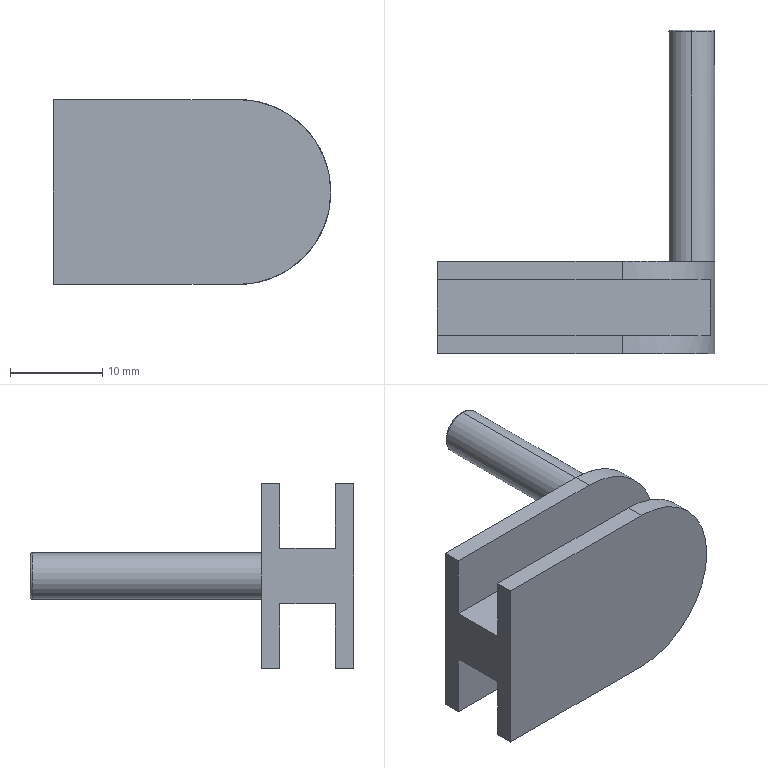Part | SolidWorks | features ICE 3, Extrusion 1, Fillet 1 | 1 solid | 19 faces | box 30 x 35 x 20 mm | volume 3794 mm3 | plane 14 | cylinder 3 | torus 2 | commonest cylinder face diameters 5 x2 20 x1
STEP:
#1=CARTESIAN_POINT('',(27.5,34.8,-12.5));
#2=VERTEX_POINT('',#1);
#3=CARTESIAN_POINT('',(27.5,34.8,-7.5));
#4=VERTEX_POINT('',#3);
#5=CARTESIAN_POINT('',(27.5,34.8,-10.));
#6=DIRECTION('',(0.,-1.,0.));
#7=DIRECTION('',(0.,0.,1.));
#8=AXIS2_PLACEMENT_3D('',#5,#6,#7);
#9=CIRCLE('',#8,2.5);
#10=EDGE_CURVE('',#2,#4,#9,.T.);
#11=ORIENTED_EDGE('',*,*,#10,.F.);
#12=CARTESIAN_POINT('',(27.5,35.,-12.3));
#13=VERTEX_POINT('',#12);
#14=CARTESIAN_POINT('',(27.5,34.8,-12.3));
#15=DIRECTION('',(1.,0.,0.));
#16=DIRECTION('',(0.,0.,-1.));
#17=AXIS2_PLACEMENT_3D('',#14,#15,#16);
#18=CIRCLE('',#17,0.2);
#19=EDGE_CURVE('',#2,#13,#18,.T.);
#20=ORIENTED_EDGE('',*,*,#19,.T.);
#21=CARTESIAN_POINT('',(27.5,35.,-7.7));
#22=VERTEX_POINT('',#21);
#23=CARTESIAN_POINT('',(27.5,35.,-10.));
#24=DIRECTION('',(0.,1.,0.));
#25=DIRECTION('',(0.,0.,1.));
#26=AXIS2_PLACEMENT_3D('',#23,#24,#25);
#27=CIRCLE('',#26,2.3);
#28=EDGE_CURVE('',#22,#13,#27,.T.);
#29=ORIENTED_EDGE('',*,*,#28,.F.);
#30=CARTESIAN_POINT('',(27.5,34.8,-7.7));
#31=DIRECTION('',(-1.,0.,0.));
#32=DIRECTION('',(0.,0.,1.));
#33=AXIS2_PLACEMENT_3D('',#30,#31,#32);
#34=CIRCLE('',#33,0.2);
#35=EDGE_CURVE('',#4,#22,#34,.T.);
#36=ORIENTED_EDGE('',*,*,#35,.F.);
#37=EDGE_LOOP('',(#11,#20,#29,#36));
#38=FACE_OUTER_BOUND('',#37,.T.);
#39=CARTESIAN_POINT('',(27.5,34.8,-10.));
#40=DIRECTION('',(0.,1.,0.));
#41=DIRECTION('',(0.,0.,1.));
#42=AXIS2_PLACEMENT_3D('',#39,#40,#41);
#43=TOROIDAL_SURFACE('',#42,2.3,0.2);
#44=ADVANCED_FACE('',(#38),#43,.T.);
#45=ORIENTED_EDGE('',*,*,#10,.T.);
#46=CARTESIAN_POINT('',(27.5,10.,-7.5));
#47=VERTEX_POINT('',#46);
#48=CARTESIAN_POINT('',(27.5,35.,-7.5));
#49=DIRECTION('',(0.,-1.,0.));
#50=VECTOR('',#49,1000.);
#51=LINE('',#48,#50);
#52=EDGE_CURVE('',#4,#47,#51,.T.);
#53=ORIENTED_EDGE('',*,*,#52,.T.);
#54=CARTESIAN_POINT('',(30.,10.,-10.));
#55=VERTEX_POINT('',#54);
#56=CARTESIAN_POINT('',(27.5,10.,-10.));
#57=DIRECTION('',(0.,1.,0.));
#58=DIRECTION('',(0.,0.,1.));
#59=AXIS2_PLACEMENT_3D('',#56,#57,#58);
#60=CIRCLE('',#59,2.5);
#61=EDGE_CURVE('',#47,#55,#60,.T.);
#62=ORIENTED_EDGE('',*,*,#61,.T.);
#63=CARTESIAN_POINT('',(27.5,10.,-12.5));
#64=VERTEX_POINT('',#63);
#65=CARTESIAN_POINT('',(27.5,10.,-10.));
#66=DIRECTION('',(0.,1.,0.));
#67=DIRECTION('',(0.,0.,1.));
#68=AXIS2_PLACEMENT_3D('',#65,#66,#67);
#69=CIRCLE('',#68,2.5);
#70=EDGE_CURVE('',#55,#64,#69,.T.);
#71=ORIENTED_EDGE('',*,*,#70,.T.);
#72=CARTESIAN_POINT('',(27.5,35.,-12.5));
#73=DIRECTION('',(0.,-1.,0.));
#74=VECTOR('',#73,1000.);
#75=LINE('',#72,#74);
#76=EDGE_CURVE('',#2,#64,#75,.T.);
#77=ORIENTED_EDGE('',*,*,#76,.F.);
#78=EDGE_LOOP('',(#45,#53,#62,#71,#77));
#79=FACE_OUTER_BOUND('',#78,.T.);
#80=CARTESIAN_POINT('',(27.5,35.,-10.));
#81=DIRECTION('',(0.,-1.,0.));
#82=DIRECTION('',(0.,0.,-1.));
#83=AXIS2_PLACEMENT_3D('',#80,#81,#82);
#84=CYLINDRICAL_SURFACE('',#83,2.5);
#85=ADVANCED_FACE('',(#79),#84,.T.);
#86=CARTESIAN_POINT('',(20.,10.,0.));
#87=VERTEX_POINT('',#86);
#88=CARTESIAN_POINT('',(20.,10.,-10.));
#89=DIRECTION('',(0.,-1.,0.));
#90=DIRECTION('',(0.,0.,1.));
#91=AXIS2_PLACEMENT_3D('',#88,#89,#90);
#92=CIRCLE('',#91,10.);
#93=EDGE_CURVE('',#55,#87,#92,.T.);
#94=ORIENTED_EDGE('',*,*,#93,.F.);
#95=ORIENTED_EDGE('',*,*,#61,.F.);
#96=CARTESIAN_POINT('',(27.5,10.,-10.));
#97=DIRECTION('',(0.,1.,0.));
#98=DIRECTION('',(0.,0.,1.));
#99=AXIS2_PLACEMENT_3D('',#96,#97,#98);
#100=CIRCLE('',#99,2.5);
#101=EDGE_CURVE('',#64,#47,#100,.T.);
#102=ORIENTED_EDGE('',*,*,#101,.F.);
#103=ORIENTED_EDGE('',*,*,#70,.F.);
#104=CARTESIAN_POINT('',(20.,10.,-20.));
#105=VERTEX_POINT('',#104);
#106=CARTESIAN_POINT('',(20.,10.,-10.));
#107=DIRECTION('',(0.,-1.,0.));
#108=DIRECTION('',(0.,0.,1.));
#109=AXIS2_PLACEMENT_3D('',#106,#107,#108);
#110=CIRCLE('',#109,10.);
#111=EDGE_CURVE('',#105,#55,#110,.T.);
#112=ORIENTED_EDGE('',*,*,#111,.F.);
#113=CARTESIAN_POINT('',(0.,10.,-20.));
#114=VERTEX_POINT('',#113);
#115=CARTESIAN_POINT('',(0.,10.,-20.));
#116=DIRECTION('',(-1.,0.,0.));
#117=VECTOR('',#116,1000.);
#118=LINE('',#115,#117);
#119=EDGE_CURVE('',#105,#114,#118,.T.);
#120=ORIENTED_EDGE('',*,*,#119,.T.);
#121=CARTESIAN_POINT('',(0.,10.,0.));
#122=VERTEX_POINT('',#121);
#123=CARTESIAN_POINT('',(0.,10.,0.));
#124=DIRECTION('',(0.,0.,1.));
#125=VECTOR('',#124,1000.);
#126=LINE('',#123,#125);
#127=EDGE_CURVE('',#114,#122,#126,.T.);
#128=ORIENTED_EDGE('',*,*,#127,.T.);
#129=CARTESIAN_POINT('',(0.,10.,0.));
#130=DIRECTION('',(1.,0.,0.));
#131=VECTOR('',#130,1000.);
#132=LINE('',#129,#131);
#133=EDGE_CURVE('',#122,#87,#132,.T.);
#134=ORIENTED_EDGE('',*,*,#133,.T.);
#135=EDGE_LOOP('',(#94,#95,#102,#103,#112,#120,#128,#134));
#136=FACE_OUTER_BOUND('',#135,.T.);
#137=CARTESIAN_POINT('',(0.,10.,0.));
#138=DIRECTION('',(0.,-1.,0.));
#139=DIRECTION('',(0.,0.,-1.));
#140=AXIS2_PLACEMENT_3D('',#137,#138,#139);
#141=PLANE('',#140);
#142=ADVANCED_FACE('',(#136),#141,.F.);
#143=CARTESIAN_POINT('',(20.,0.,0.));
#144=VERTEX_POINT('',#143);
#145=CARTESIAN_POINT('',(20.,2.,0.));
#146=VERTEX_POINT('',#145);
#147=CARTESIAN_POINT('',(20.,0.,0.));
#148=DIRECTION('',(0.,1.,0.));
#149=VECTOR('',#148,1000.);
#150=LINE('',#147,#149);
#151=EDGE_CURVE('',#144,#146,#150,.T.);
#152=ORIENTED_EDGE('',*,*,#151,.T.);
#153=CARTESIAN_POINT('',(0.,2.,0.));
#154=VERTEX_POINT('',#153);
#155=CARTESIAN_POINT('',(30.,2.,0.));
#156=DIRECTION('',(-1.,0.,0.));
#157=VECTOR('',#156,1000.);
#158=LINE('',#155,#157);
#159=EDGE_CURVE('',#146,#154,#158,.T.);
#160=ORIENTED_EDGE('',*,*,#159,.T.);
#161=CARTESIAN_POINT('',(0.,0.,0.));
#162=VERTEX_POINT('',#161);
#163=CARTESIAN_POINT('',(0.,10.,0.));
#164=DIRECTION('',(0.,-1.,0.));
#165=VECTOR('',#164,1000.);
#166=LINE('',#163,#165);
#167=EDGE_CURVE('',#154,#162,#166,.T.);
#168=ORIENTED_EDGE('',*,*,#167,.T.);
#169=CARTESIAN_POINT('',(0.,0.,0.));
#170=DIRECTION('',(1.,0.,0.));
#171=VECTOR('',#170,1000.);
#172=LINE('',#169,#171);
#173=EDGE_CURVE('',#162,#144,#172,.T.);
#174=ORIENTED_EDGE('',*,*,#173,.T.);
#175=EDGE_LOOP('',(#152,#160,#168,#174));
#176=FACE_OUTER_BOUND('',#175,.T.);
#177=CARTESIAN_POINT('',(0.,10.,0.));
#178=DIRECTION('',(0.,0.,-1.));
#179=DIRECTION('',(-1.,0.,0.));
#180=AXIS2_PLACEMENT_3D('',#177,#178,#179);
#181=PLANE('',#180);
#182=ADVANCED_FACE('',(#176),#181,.F.);
#183=CARTESIAN_POINT('',(20.,8.,0.));
#184=VERTEX_POINT('',#183);
#185=CARTESIAN_POINT('',(20.,0.,0.));
#186=DIRECTION('',(0.,1.,0.));
#187=VECTOR('',#186,1000.);
#188=LINE('',#185,#187);
#189=EDGE_CURVE('',#184,#87,#188,.T.);
#190=ORIENTED_EDGE('',*,*,#189,.T.);
#191=ORIENTED_EDGE('',*,*,#133,.F.);
#192=CARTESIAN_POINT('',(0.,8.,0.));
#193=VERTEX_POINT('',#192);
#194=CARTESIAN_POINT('',(0.,10.,0.));
#195=DIRECTION('',(0.,-1.,0.));
#196=VECTOR('',#195,1000.);
#197=LINE('',#194,#196);
#198=EDGE_CURVE('',#122,#193,#197,.T.);
#199=ORIENTED_EDGE('',*,*,#198,.T.);
#200=CARTESIAN_POINT('',(30.,8.,0.));
#201=DIRECTION('',(-1.,0.,0.));
#202=VECTOR('',#201,1000.);
#203=LINE('',#200,#202);
#204=EDGE_CURVE('',#184,#193,#203,.T.);
#205=ORIENTED_EDGE('',*,*,#204,.F.);
#206=EDGE_LOOP('',(#190,#191,#199,#205));
#207=FACE_OUTER_BOUND('',#206,.T.);
#208=CARTESIAN_POINT('',(0.,10.,0.));
#209=DIRECTION('',(0.,0.,-1.));
#210=DIRECTION('',(-1.,0.,0.));
#211=AXIS2_PLACEMENT_3D('',#208,#209,#210);
#212=PLANE('',#211);
#213=ADVANCED_FACE('',(#207),#212,.F.);
#214=ORIENTED_EDGE('',*,*,#119,.F.);
#215=CARTESIAN_POINT('',(20.,8.,-20.));
#216=VERTEX_POINT('',#215);
#217=CARTESIAN_POINT('',(20.,0.,-20.));
#218=DIRECTION('',(0.,1.,0.));
#219=VECTOR('',#218,1000.);
#220=LINE('',#217,#219);
#221=EDGE_CURVE('',#216,#105,#220,.T.);
#222=ORIENTED_EDGE('',*,*,#221,.F.);
#223=CARTESIAN_POINT('',(0.,8.,-20.));
#224=VERTEX_POINT('',#223);
#225=CARTESIAN_POINT('',(30.,8.,-20.));
#226=DIRECTION('',(-1.,0.,0.));
#227=VECTOR('',#226,1000.);
#228=LINE('',#225,#227);
#229=EDGE_CURVE('',#216,#224,#228,.T.);
#230=ORIENTED_EDGE('',*,*,#229,.T.);
#231=CARTESIAN_POINT('',(0.,10.,-20.));
#232=DIRECTION('',(0.,-1.,0.));
#233=VECTOR('',#232,1000.);
#234=LINE('',#231,#233);
#235=EDGE_CURVE('',#114,#224,#234,.T.);
#236=ORIENTED_EDGE('',*,*,#235,.F.);
#237=EDGE_LOOP('',(#214,#222,#230,#236));
#238=FACE_OUTER_BOUND('',#237,.T.);
#239=CARTESIAN_POINT('',(0.,10.,-20.));
#240=DIRECTION('',(0.,0.,1.));
#241=DIRECTION('',(1.,0.,0.));
#242=AXIS2_PLACEMENT_3D('',#239,#240,#241);
#243=PLANE('',#242);
#244=ADVANCED_FACE('',(#238),#243,.F.);
#245=ORIENTED_EDGE('',*,*,#167,.F.);
#246=CARTESIAN_POINT('',(0.,2.,-7.));
#247=VERTEX_POINT('',#246);
#248=CARTESIAN_POINT('',(0.,2.,-7.));
#249=DIRECTION('',(0.,0.,1.));
#250=VECTOR('',#249,1000.);
#251=LINE('',#248,#250);
#252=EDGE_CURVE('',#247,#154,#251,.T.);
#253=ORIENTED_EDGE('',*,*,#252,.F.);
#254=CARTESIAN_POINT('',(0.,8.,-7.));
#255=VERTEX_POINT('',#254);
#256=CARTESIAN_POINT('',(0.,8.,-7.));
#257=DIRECTION('',(0.,-1.,0.));
#258=VECTOR('',#257,1000.);
#259=LINE('',#256,#258);
#260=EDGE_CURVE('',#255,#247,#259,.T.);
#261=ORIENTED_EDGE('',*,*,#260,.F.);
#262=CARTESIAN_POINT('',(0.,8.,-7.));
#263=DIRECTION('',(0.,0.,-1.));
#264=VECTOR('',#263,1000.);
#265=LINE('',#262,#264);
#266=EDGE_CURVE('',#193,#255,#265,.T.);
#267=ORIENTED_EDGE('',*,*,#266,.F.);
#268=ORIENTED_EDGE('',*,*,#198,.F.);
#269=ORIENTED_EDGE('',*,*,#127,.F.);
#270=ORIENTED_EDGE('',*,*,#235,.T.);
#271=CARTESIAN_POINT('',(0.,8.,-13.));
#272=VERTEX_POINT('',#271);
#273=CARTESIAN_POINT('',(0.,8.,-20.));
#274=DIRECTION('',(0.,0.,-1.));
#275=VECTOR('',#274,1000.);
#276=LINE('',#273,#275);
#277=EDGE_CURVE('',#272,#224,#276,.T.);
#278=ORIENTED_EDGE('',*,*,#277,.F.);
#279=CARTESIAN_POINT('',(0.,2.,-13.));
#280=VERTEX_POINT('',#279);
#281=CARTESIAN_POINT('',(0.,8.,-13.));
#282=DIRECTION('',(0.,1.,0.));
#283=VECTOR('',#282,1000.);
#284=LINE('',#281,#283);
#285=EDGE_CURVE('',#280,#272,#284,.T.);
#286=ORIENTED_EDGE('',*,*,#285,.F.);
#287=CARTESIAN_POINT('',(0.,2.,-20.));
#288=VERTEX_POINT('',#287);
#289=CARTESIAN_POINT('',(0.,2.,-20.));
#290=DIRECTION('',(0.,0.,1.));
#291=VECTOR('',#290,1000.);
#292=LINE('',#289,#291);
#293=EDGE_CURVE('',#288,#280,#292,.T.);
#294=ORIENTED_EDGE('',*,*,#293,.F.);
#295=CARTESIAN_POINT('',(0.,0.,-20.));
#296=VERTEX_POINT('',#295);
#297=CARTESIAN_POINT('',(0.,10.,-20.));
#298=DIRECTION('',(0.,-1.,0.));
#299=VECTOR('',#298,1000.);
#300=LINE('',#297,#299);
#301=EDGE_CURVE('',#288,#296,#300,.T.);
#302=ORIENTED_EDGE('',*,*,#301,.T.);
#303=CARTESIAN_POINT('',(0.,0.,0.));
#304=DIRECTION('',(0.,0.,1.));
#305=VECTOR('',#304,1000.);
#306=LINE('',#303,#305);
#307=EDGE_CURVE('',#296,#162,#306,.T.);
#308=ORIENTED_EDGE('',*,*,#307,.T.);
#309=EDGE_LOOP('',(#245,#253,#261,#267,#268,#269,#270,#278,#286,#294,#302,#308));
#310=FACE_OUTER_BOUND('',#309,.T.);
#311=CARTESIAN_POINT('',(0.,10.,0.));
#312=DIRECTION('',(1.,0.,0.));
#313=DIRECTION('',(0.,0.,-1.));
#314=AXIS2_PLACEMENT_3D('',#311,#312,#313);
#315=PLANE('',#314);
#316=ADVANCED_FACE('',(#310),#315,.F.);
#317=CARTESIAN_POINT('',(20.,2.,-20.));
#318=VERTEX_POINT('',#317);
#319=CARTESIAN_POINT('',(30.,2.,-20.));
#320=DIRECTION('',(-1.,0.,0.));
#321=VECTOR('',#320,1000.);
#322=LINE('',#319,#321);
#323=EDGE_CURVE('',#318,#288,#322,.T.);
#324=ORIENTED_EDGE('',*,*,#323,.F.);
#325=CARTESIAN_POINT('',(20.,0.,-20.));
#326=VERTEX_POINT('',#325);
#327=CARTESIAN_POINT('',(20.,0.,-20.));
#328=DIRECTION('',(0.,1.,0.));
#329=VECTOR('',#328,1000.);
#330=LINE('',#327,#329);
#331=EDGE_CURVE('',#326,#318,#330,.T.);
#332=ORIENTED_EDGE('',*,*,#331,.F.);
#333=CARTESIAN_POINT('',(0.,0.,-20.));
#334=DIRECTION('',(-1.,0.,0.));
#335=VECTOR('',#334,1000.);
#336=LINE('',#333,#335);
#337=EDGE_CURVE('',#326,#296,#336,.T.);
#338=ORIENTED_EDGE('',*,*,#337,.T.);
#339=ORIENTED_EDGE('',*,*,#301,.F.);
#340=EDGE_LOOP('',(#324,#332,#338,#339));
#341=FACE_OUTER_BOUND('',#340,.T.);
#342=CARTESIAN_POINT('',(0.,10.,-20.));
#343=DIRECTION('',(0.,0.,1.));
#344=DIRECTION('',(1.,0.,0.));
#345=AXIS2_PLACEMENT_3D('',#342,#343,#344);
#346=PLANE('',#345);
#347=ADVANCED_FACE('',(#341),#346,.F.);
#348=ORIENTED_EDGE('',*,*,#337,.F.);
#349=CARTESIAN_POINT('',(20.,0.,-10.));
#350=DIRECTION('',(0.,-1.,0.));
#351=DIRECTION('',(0.,0.,1.));
#352=AXIS2_PLACEMENT_3D('',#349,#350,#351);
#353=CIRCLE('',#352,10.);
#354=EDGE_CURVE('',#326,#144,#353,.T.);
#355=ORIENTED_EDGE('',*,*,#354,.T.);
#356=ORIENTED_EDGE('',*,*,#173,.F.);
#357=ORIENTED_EDGE('',*,*,#307,.F.);
#358=EDGE_LOOP('',(#348,#355,#356,#357));
#359=FACE_OUTER_BOUND('',#358,.T.);
#360=CARTESIAN_POINT('',(0.,0.,0.));
#361=DIRECTION('',(0.,-1.,0.));
#362=DIRECTION('',(0.,0.,-1.));
#363=AXIS2_PLACEMENT_3D('',#360,#361,#362);
#364=PLANE('',#363);
#365=ADVANCED_FACE('',(#359),#364,.T.);
#366=ORIENTED_EDGE('',*,*,#229,.F.);
#367=CARTESIAN_POINT('',(29.539,8.,-13.));
#368=VERTEX_POINT('',#367);
#369=CARTESIAN_POINT('',(20.,8.,-10.));
#370=DIRECTION('',(0.,-1.,0.));
#371=DIRECTION('',(0.,0.,1.));
#372=AXIS2_PLACEMENT_3D('',#369,#370,#371);
#373=CIRCLE('',#372,10.);
#374=EDGE_CURVE('',#216,#368,#373,.T.);
#375=ORIENTED_EDGE('',*,*,#374,.T.);
#376=CARTESIAN_POINT('',(30.,8.,-13.));
#377=DIRECTION('',(-1.,0.,0.));
#378=VECTOR('',#377,1000.);
#379=LINE('',#376,#378);
#380=EDGE_CURVE('',#368,#272,#379,.T.);
#381=ORIENTED_EDGE('',*,*,#380,.T.);
#382=ORIENTED_EDGE('',*,*,#277,.T.);
#383=EDGE_LOOP('',(#366,#375,#381,#382));
#384=FACE_OUTER_BOUND('',#383,.T.);
#385=CARTESIAN_POINT('',(30.,8.,-20.));
#386=DIRECTION('',(0.,1.,0.));
#387=DIRECTION('',(0.,0.,1.));
#388=AXIS2_PLACEMENT_3D('',#385,#386,#387);
#389=PLANE('',#388);
#390=ADVANCED_FACE('',(#384),#389,.F.);
#391=ORIENTED_EDGE('',*,*,#380,.F.);
#392=CARTESIAN_POINT('',(29.539,2.,-13.));
#393=VERTEX_POINT('',#392);
#394=CARTESIAN_POINT('',(29.539,0.,-13.));
#395=DIRECTION('',(0.,-1.,0.));
#396=VECTOR('',#395,1000.);
#397=LINE('',#394,#396);
#398=EDGE_CURVE('',#368,#393,#397,.T.);
#399=ORIENTED_EDGE('',*,*,#398,.T.);
#400=CARTESIAN_POINT('',(30.,2.,-13.));
#401=DIRECTION('',(-1.,0.,0.));
#402=VECTOR('',#401,1000.);
#403=LINE('',#400,#402);
#404=EDGE_CURVE('',#393,#280,#403,.T.);
#405=ORIENTED_EDGE('',*,*,#404,.T.);
#406=ORIENTED_EDGE('',*,*,#285,.T.);
#407=EDGE_LOOP('',(#391,#399,#405,#406));
#408=FACE_OUTER_BOUND('',#407,.T.);
#409=CARTESIAN_POINT('',(30.,8.,-13.));
#410=DIRECTION('',(0.,0.,1.));
#411=DIRECTION('',(1.,0.,0.));
#412=AXIS2_PLACEMENT_3D('',#409,#410,#411);
#413=PLANE('',#412);
#414=ADVANCED_FACE('',(#408),#413,.F.);
#415=ORIENTED_EDGE('',*,*,#404,.F.);
#416=CARTESIAN_POINT('',(20.,2.,-10.));
#417=DIRECTION('',(0.,1.,0.));
#418=DIRECTION('',(0.,0.,-1.));
#419=AXIS2_PLACEMENT_3D('',#416,#417,#418);
#420=CIRCLE('',#419,10.);
#421=EDGE_CURVE('',#393,#318,#420,.T.);
#422=ORIENTED_EDGE('',*,*,#421,.T.);
#423=ORIENTED_EDGE('',*,*,#323,.T.);
#424=ORIENTED_EDGE('',*,*,#293,.T.);
#425=EDGE_LOOP('',(#415,#422,#423,#424));
#426=FACE_OUTER_BOUND('',#425,.T.);
#427=CARTESIAN_POINT('',(30.,2.,-20.));
#428=DIRECTION('',(0.,-1.,0.));
#429=DIRECTION('',(0.,0.,-1.));
#430=AXIS2_PLACEMENT_3D('',#427,#428,#429);
#431=PLANE('',#430);
#432=ADVANCED_FACE('',(#426),#431,.F.);
#433=ORIENTED_EDGE('',*,*,#159,.F.);
#434=CARTESIAN_POINT('',(29.539,2.,-7.));
#435=VERTEX_POINT('',#434);
#436=CARTESIAN_POINT('',(20.,2.,-10.));
#437=DIRECTION('',(0.,1.,0.));
#438=DIRECTION('',(0.,0.,-1.));
#439=AXIS2_PLACEMENT_3D('',#436,#437,#438);
#440=CIRCLE('',#439,10.);
#441=EDGE_CURVE('',#146,#435,#440,.T.);
#442=ORIENTED_EDGE('',*,*,#441,.T.);
#443=CARTESIAN_POINT('',(30.,2.,-7.));
#444=DIRECTION('',(-1.,0.,0.));
#445=VECTOR('',#444,1000.);
#446=LINE('',#443,#445);
#447=EDGE_CURVE('',#435,#247,#446,.T.);
#448=ORIENTED_EDGE('',*,*,#447,.T.);
#449=ORIENTED_EDGE('',*,*,#252,.T.);
#450=EDGE_LOOP('',(#433,#442,#448,#449));
#451=FACE_OUTER_BOUND('',#450,.T.);
#452=CARTESIAN_POINT('',(30.,2.,-7.));
#453=DIRECTION('',(0.,-1.,0.));
#454=DIRECTION('',(0.,0.,-1.));
#455=AXIS2_PLACEMENT_3D('',#452,#453,#454);
#456=PLANE('',#455);
#457=ADVANCED_FACE('',(#451),#456,.F.);
#458=ORIENTED_EDGE('',*,*,#447,.F.);
#459=CARTESIAN_POINT('',(29.539,8.,-7.));
#460=VERTEX_POINT('',#459);
#461=CARTESIAN_POINT('',(29.539,0.,-7.));
#462=DIRECTION('',(0.,1.,0.));
#463=VECTOR('',#462,1000.);
#464=LINE('',#461,#463);
#465=EDGE_CURVE('',#435,#460,#464,.T.);
#466=ORIENTED_EDGE('',*,*,#465,.T.);
#467=CARTESIAN_POINT('',(30.,8.,-7.));
#468=DIRECTION('',(-1.,0.,0.));
#469=VECTOR('',#468,1000.);
#470=LINE('',#467,#469);
#471=EDGE_CURVE('',#460,#255,#470,.T.);
#472=ORIENTED_EDGE('',*,*,#471,.T.);
#473=ORIENTED_EDGE('',*,*,#260,.T.);
#474=EDGE_LOOP('',(#458,#466,#472,#473));
#475=FACE_OUTER_BOUND('',#474,.T.);
#476=CARTESIAN_POINT('',(30.,8.,-7.));
#477=DIRECTION('',(0.,0.,-1.));
#478=DIRECTION('',(-1.,0.,0.));
#479=AXIS2_PLACEMENT_3D('',#476,#477,#478);
#480=PLANE('',#479);
#481=ADVANCED_FACE('',(#475),#480,.F.);
#482=ORIENTED_EDGE('',*,*,#471,.F.);
#483=CARTESIAN_POINT('',(20.,8.,-10.));
#484=DIRECTION('',(0.,-1.,0.));
#485=DIRECTION('',(0.,0.,1.));
#486=AXIS2_PLACEMENT_3D('',#483,#484,#485);
#487=CIRCLE('',#486,10.);
#488=EDGE_CURVE('',#460,#184,#487,.T.);
#489=ORIENTED_EDGE('',*,*,#488,.T.);
#490=ORIENTED_EDGE('',*,*,#204,.T.);
#491=ORIENTED_EDGE('',*,*,#266,.T.);
#492=EDGE_LOOP('',(#482,#489,#490,#491));
#493=FACE_OUTER_BOUND('',#492,.T.);
#494=CARTESIAN_POINT('',(30.,8.,-7.));
#495=DIRECTION('',(0.,1.,0.));
#496=DIRECTION('',(0.,0.,1.));
#497=AXIS2_PLACEMENT_3D('',#494,#495,#496);
#498=PLANE('',#497);
#499=ADVANCED_FACE('',(#493),#498,.F.);
#500=ORIENTED_EDGE('',*,*,#151,.F.);
#501=ORIENTED_EDGE('',*,*,#354,.F.);
#502=ORIENTED_EDGE('',*,*,#331,.T.);
#503=ORIENTED_EDGE('',*,*,#421,.F.);
#504=ORIENTED_EDGE('',*,*,#398,.F.);
#505=ORIENTED_EDGE('',*,*,#374,.F.);
#506=ORIENTED_EDGE('',*,*,#221,.T.);
#507=ORIENTED_EDGE('',*,*,#111,.T.);
#508=ORIENTED_EDGE('',*,*,#93,.T.);
#509=ORIENTED_EDGE('',*,*,#189,.F.);
#510=ORIENTED_EDGE('',*,*,#488,.F.);
#511=ORIENTED_EDGE('',*,*,#465,.F.);
#512=ORIENTED_EDGE('',*,*,#441,.F.);
#513=EDGE_LOOP('',(#500,#501,#502,#503,#504,#505,#506,#507,#508,#509,#510,#511,#512));
#514=FACE_OUTER_BOUND('',#513,.T.);
#515=CARTESIAN_POINT('',(20.,0.,-10.));
#516=DIRECTION('',(0.,1.,0.));
#517=DIRECTION('',(0.,0.,1.));
#518=AXIS2_PLACEMENT_3D('',#515,#516,#517);
#519=CYLINDRICAL_SURFACE('',#518,10.);
#520=ADVANCED_FACE('',(#514),#519,.T.);
#521=ORIENTED_EDGE('',*,*,#52,.F.);
#522=CARTESIAN_POINT('',(27.5,34.8,-10.));
#523=DIRECTION('',(0.,-1.,0.));
#524=DIRECTION('',(0.,0.,1.));
#525=AXIS2_PLACEMENT_3D('',#522,#523,#524);
#526=CIRCLE('',#525,2.5);
#527=EDGE_CURVE('',#4,#2,#526,.T.);
#528=ORIENTED_EDGE('',*,*,#527,.T.);
#529=ORIENTED_EDGE('',*,*,#76,.T.);
#530=ORIENTED_EDGE('',*,*,#101,.T.);
#531=EDGE_LOOP('',(#521,#528,#529,#530));
#532=FACE_OUTER_BOUND('',#531,.T.);
#533=CARTESIAN_POINT('',(27.5,35.,-10.));
#534=DIRECTION('',(0.,-1.,0.));
#535=DIRECTION('',(0.,0.,-1.));
#536=AXIS2_PLACEMENT_3D('',#533,#534,#535);
#537=CYLINDRICAL_SURFACE('',#536,2.5);
#538=ADVANCED_FACE('',(#532),#537,.T.);
#539=ORIENTED_EDGE('',*,*,#28,.T.);
#540=CARTESIAN_POINT('',(27.5,35.,-10.));
#541=DIRECTION('',(0.,1.,0.));
#542=DIRECTION('',(0.,0.,1.));
#543=AXIS2_PLACEMENT_3D('',#540,#541,#542);
#544=CIRCLE('',#543,2.3);
#545=EDGE_CURVE('',#13,#22,#544,.T.);
#546=ORIENTED_EDGE('',*,*,#545,.T.);
#547=EDGE_LOOP('',(#539,#546));
#548=FACE_OUTER_BOUND('',#547,.T.);
#549=CARTESIAN_POINT('',(27.5,35.,-10.));
#550=DIRECTION('',(0.,1.,0.));
#551=DIRECTION('',(0.,0.,1.));
#552=AXIS2_PLACEMENT_3D('',#549,#550,#551);
#553=PLANE('',#552);
#554=ADVANCED_FACE('',(#548),#553,.T.);
#555=ORIENTED_EDGE('',*,*,#19,.F.);
#556=ORIENTED_EDGE('',*,*,#527,.F.);
#557=ORIENTED_EDGE('',*,*,#35,.T.);
#558=ORIENTED_EDGE('',*,*,#545,.F.);
#559=EDGE_LOOP('',(#555,#556,#557,#558));
#560=FACE_OUTER_BOUND('',#559,.T.);
#561=CARTESIAN_POINT('',(27.5,34.8,-10.));
#562=DIRECTION('',(0.,1.,0.));
#563=DIRECTION('',(0.,0.,1.));
#564=AXIS2_PLACEMENT_3D('',#561,#562,#563);
#565=TOROIDAL_SURFACE('',#564,2.3,0.2);
#566=ADVANCED_FACE('',(#560),#565,.T.);
#567=CLOSED_SHELL('',(#44,#85,#142,#182,#213,#244,#316,#347,#365,#390,#414,#432,#457,#481,#499,#520,#538,#554,#566));
#568=MANIFOLD_SOLID_BREP('',#567);
#569=CARTESIAN_POINT('',(0.,0.,0.));
#570=DIRECTION('',(0.,0.,1.));
#571=DIRECTION('',(1.,0.,0.));
#572=AXIS2_PLACEMENT_3D('',#569,#570,#571);
#573=(LENGTH_UNIT()NAMED_UNIT(*)SI_UNIT(.MILLI.,.METRE.));
#574=UNCERTAINTY_MEASURE_WITH_UNIT(LENGTH_MEASURE(0.00001),#573,'','');
#575=(NAMED_UNIT(*)PLANE_ANGLE_UNIT()SI_UNIT($,.RADIAN.));
#576=(NAMED_UNIT(*)SI_UNIT($,.STERADIAN.)SOLID_ANGLE_UNIT());
#577=(GEOMETRIC_REPRESENTATION_CONTEXT(3)GLOBAL_UNCERTAINTY_ASSIGNED_CONTEXT((#574))GLOBAL_UNIT_ASSIGNED_CONTEXT((#573,#575,#576))REPRESENTATION_CONTEXT('',''));
#578=ADVANCED_BREP_SHAPE_REPRESENTATION('',(#568,#572),#577);